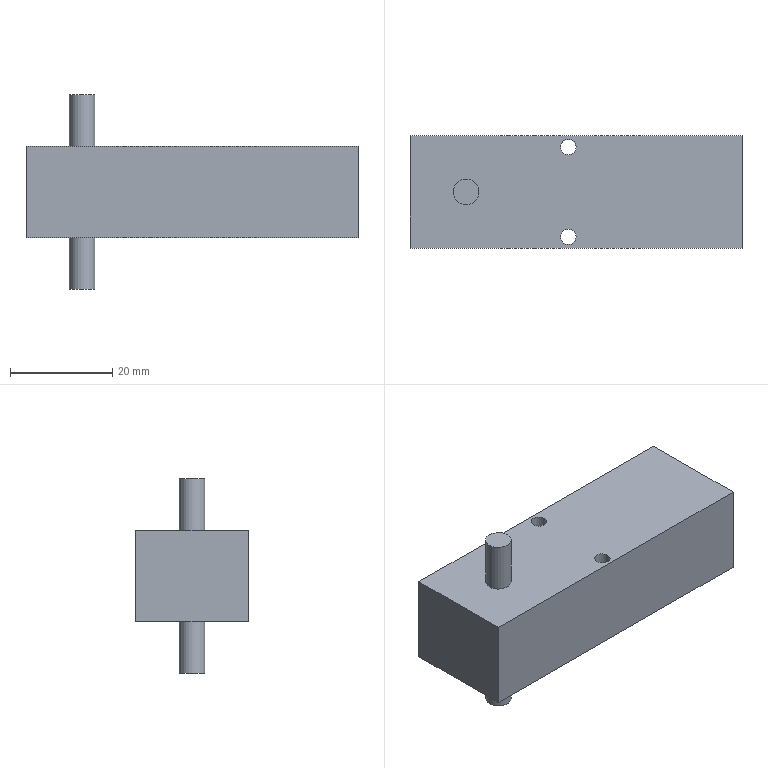Part | NX | features BREP 1 | 1 solid | 12 faces | box 65 x 22 x 38 mm | volume 25878 mm3 | plane 8 | cylinder 4 | commonest cylinder face diameters 3 x2 5 x2
STEP:
#1=CARTESIAN_POINT('',(-3.,-8.8,9.));
#2=VERTEX_POINT('',#1);
#3=CARTESIAN_POINT('',(-1.5,-8.8,9.));
#4=DIRECTION('',(0.,0.,1.));
#5=DIRECTION('',(-1.,0.,0.));
#6=AXIS2_PLACEMENT_3D('',#3,#4,#5);
#7=CIRCLE('',#6,1.5);
#8=EDGE_CURVE('',#2,#2,#7,.T.);
#9=ORIENTED_EDGE('',*,*,#8,.T.);
#10=EDGE_LOOP('',(#9));
#11=FACE_BOUND('',#10,.T.);
#12=CARTESIAN_POINT('',(0.,-8.8,-9.));
#13=VERTEX_POINT('',#12);
#14=CARTESIAN_POINT('',(-1.5,-8.8,-9.));
#15=DIRECTION('',(0.,0.,-1.));
#16=DIRECTION('',(1.,0.,0.));
#17=AXIS2_PLACEMENT_3D('',#14,#15,#16);
#18=CIRCLE('',#17,1.5);
#19=EDGE_CURVE('',#13,#13,#18,.T.);
#20=ORIENTED_EDGE('',*,*,#19,.T.);
#21=EDGE_LOOP('',(#20));
#22=FACE_BOUND('',#21,.T.);
#23=CARTESIAN_POINT('',(-1.5,-8.8,-13.243));
#24=DIRECTION('',(0.,0.,1.));
#25=DIRECTION('',(-1.,0.,0.));
#26=AXIS2_PLACEMENT_3D('',#23,#24,#25);
#27=CYLINDRICAL_SURFACE('',#26,1.5);
#28=ADVANCED_FACE('',(#11,#22),#27,.F.);
#29=CARTESIAN_POINT('',(0.,8.8,9.));
#30=VERTEX_POINT('',#29);
#31=CARTESIAN_POINT('',(-1.5,8.8,9.));
#32=DIRECTION('',(0.,0.,1.));
#33=DIRECTION('',(1.,0.,0.));
#34=AXIS2_PLACEMENT_3D('',#31,#32,#33);
#35=CIRCLE('',#34,1.5);
#36=EDGE_CURVE('',#30,#30,#35,.T.);
#37=ORIENTED_EDGE('',*,*,#36,.T.);
#38=EDGE_LOOP('',(#37));
#39=FACE_BOUND('',#38,.T.);
#40=CARTESIAN_POINT('',(0.,8.8,-9.));
#41=VERTEX_POINT('',#40);
#42=CARTESIAN_POINT('',(-1.5,8.8,-9.));
#43=DIRECTION('',(0.,0.,-1.));
#44=DIRECTION('',(1.,0.,0.));
#45=AXIS2_PLACEMENT_3D('',#42,#43,#44);
#46=CIRCLE('',#45,1.5);
#47=EDGE_CURVE('',#41,#41,#46,.T.);
#48=ORIENTED_EDGE('',*,*,#47,.T.);
#49=EDGE_LOOP('',(#48));
#50=FACE_BOUND('',#49,.T.);
#51=CARTESIAN_POINT('',(-1.5,8.8,-13.243));
#52=DIRECTION('',(0.,0.,1.));
#53=DIRECTION('',(-1.,0.,0.));
#54=AXIS2_PLACEMENT_3D('',#51,#52,#53);
#55=CYLINDRICAL_SURFACE('',#54,1.5);
#56=ADVANCED_FACE('',(#39,#50),#55,.F.);
#57=CARTESIAN_POINT('',(-19.,0.,-9.));
#58=VERTEX_POINT('',#57);
#59=CARTESIAN_POINT('',(-21.5,0.,-9.));
#60=DIRECTION('',(0.,0.,1.));
#61=DIRECTION('',(1.,0.,0.));
#62=AXIS2_PLACEMENT_3D('',#59,#60,#61);
#63=CIRCLE('',#62,2.5);
#64=EDGE_CURVE('',#58,#58,#63,.T.);
#65=ORIENTED_EDGE('',*,*,#64,.F.);
#66=EDGE_LOOP('',(#65));
#67=FACE_BOUND('',#66,.T.);
#68=CARTESIAN_POINT('',(-19.,0.,-19.));
#69=VERTEX_POINT('',#68);
#70=CARTESIAN_POINT('',(-21.5,0.,-19.));
#71=DIRECTION('',(0.,0.,1.));
#72=DIRECTION('',(1.,0.,0.));
#73=AXIS2_PLACEMENT_3D('',#70,#71,#72);
#74=CIRCLE('',#73,2.5);
#75=EDGE_CURVE('',#69,#69,#74,.T.);
#76=ORIENTED_EDGE('',*,*,#75,.T.);
#77=EDGE_LOOP('',(#76));
#78=FACE_BOUND('',#77,.T.);
#79=CARTESIAN_POINT('',(-21.5,0.,-19.));
#80=DIRECTION('',(0.,0.,1.));
#81=DIRECTION('',(-1.,0.,0.));
#82=AXIS2_PLACEMENT_3D('',#79,#80,#81);
#83=CYLINDRICAL_SURFACE('',#82,2.5);
#84=ADVANCED_FACE('',(#67,#78),#83,.T.);
#85=CARTESIAN_POINT('',(-19.,0.,9.));
#86=VERTEX_POINT('',#85);
#87=CARTESIAN_POINT('',(-21.5,0.,9.));
#88=DIRECTION('',(0.,0.,1.));
#89=DIRECTION('',(1.,0.,0.));
#90=AXIS2_PLACEMENT_3D('',#87,#88,#89);
#91=CIRCLE('',#90,2.5);
#92=EDGE_CURVE('',#86,#86,#91,.T.);
#93=ORIENTED_EDGE('',*,*,#92,.T.);
#94=EDGE_LOOP('',(#93));
#95=FACE_BOUND('',#94,.T.);
#96=CARTESIAN_POINT('',(-19.,0.,19.));
#97=VERTEX_POINT('',#96);
#98=CARTESIAN_POINT('',(-21.5,0.,19.));
#99=DIRECTION('',(0.,0.,1.));
#100=DIRECTION('',(1.,0.,0.));
#101=AXIS2_PLACEMENT_3D('',#98,#99,#100);
#102=CIRCLE('',#101,2.5);
#103=EDGE_CURVE('',#97,#97,#102,.T.);
#104=ORIENTED_EDGE('',*,*,#103,.F.);
#105=EDGE_LOOP('',(#104));
#106=FACE_BOUND('',#105,.T.);
#107=CARTESIAN_POINT('',(-21.5,0.,19.));
#108=DIRECTION('',(0.,0.,-1.));
#109=DIRECTION('',(1.,0.,0.));
#110=AXIS2_PLACEMENT_3D('',#107,#108,#109);
#111=CYLINDRICAL_SURFACE('',#110,2.5);
#112=ADVANCED_FACE('',(#95,#106),#111,.T.);
#113=ORIENTED_EDGE('',*,*,#8,.F.);
#114=EDGE_LOOP('',(#113));
#115=FACE_BOUND('',#114,.T.);
#116=ORIENTED_EDGE('',*,*,#36,.F.);
#117=EDGE_LOOP('',(#116));
#118=FACE_BOUND('',#117,.T.);
#119=CARTESIAN_POINT('',(32.5,-11.,9.));
#120=VERTEX_POINT('',#119);
#121=CARTESIAN_POINT('',(32.5,11.,9.));
#122=VERTEX_POINT('',#121);
#123=CARTESIAN_POINT('',(32.5,11.,9.));
#124=DIRECTION('',(0.,1.,0.));
#125=VECTOR('',#124,1000.);
#126=LINE('',#123,#125);
#127=EDGE_CURVE('',#120,#122,#126,.T.);
#128=ORIENTED_EDGE('',*,*,#127,.T.);
#129=CARTESIAN_POINT('',(-32.5,11.,9.));
#130=VERTEX_POINT('',#129);
#131=CARTESIAN_POINT('',(-32.5,11.,9.));
#132=DIRECTION('',(-1.,0.,0.));
#133=VECTOR('',#132,1000.);
#134=LINE('',#131,#133);
#135=EDGE_CURVE('',#122,#130,#134,.T.);
#136=ORIENTED_EDGE('',*,*,#135,.T.);
#137=CARTESIAN_POINT('',(-32.5,-11.,9.));
#138=VERTEX_POINT('',#137);
#139=CARTESIAN_POINT('',(-32.5,11.,9.));
#140=DIRECTION('',(0.,-1.,0.));
#141=VECTOR('',#140,1000.);
#142=LINE('',#139,#141);
#143=EDGE_CURVE('',#130,#138,#142,.T.);
#144=ORIENTED_EDGE('',*,*,#143,.T.);
#145=CARTESIAN_POINT('',(-32.5,-11.,9.));
#146=DIRECTION('',(1.,0.,0.));
#147=VECTOR('',#146,1000.);
#148=LINE('',#145,#147);
#149=EDGE_CURVE('',#138,#120,#148,.T.);
#150=ORIENTED_EDGE('',*,*,#149,.T.);
#151=EDGE_LOOP('',(#128,#136,#144,#150));
#152=FACE_BOUND('',#151,.T.);
#153=ORIENTED_EDGE('',*,*,#92,.F.);
#154=EDGE_LOOP('',(#153));
#155=FACE_BOUND('',#154,.T.);
#156=CARTESIAN_POINT('',(0.,0.,9.));
#157=DIRECTION('',(0.,0.,1.));
#158=DIRECTION('',(-1.,0.,0.));
#159=AXIS2_PLACEMENT_3D('',#156,#157,#158);
#160=PLANE('',#159);
#161=ADVANCED_FACE('',(#115,#118,#152,#155),#160,.T.);
#162=CARTESIAN_POINT('',(32.5,-11.,-9.));
#163=VERTEX_POINT('',#162);
#164=CARTESIAN_POINT('',(32.5,11.,-9.));
#165=VERTEX_POINT('',#164);
#166=CARTESIAN_POINT('',(32.5,11.,-9.));
#167=DIRECTION('',(0.,1.,0.));
#168=VECTOR('',#167,1000.);
#169=LINE('',#166,#168);
#170=EDGE_CURVE('',#163,#165,#169,.T.);
#171=ORIENTED_EDGE('',*,*,#170,.T.);
#172=CARTESIAN_POINT('',(32.5,11.,9.));
#173=DIRECTION('',(0.,0.,-1.));
#174=VECTOR('',#173,1000.);
#175=LINE('',#172,#174);
#176=EDGE_CURVE('',#122,#165,#175,.T.);
#177=ORIENTED_EDGE('',*,*,#176,.F.);
#178=ORIENTED_EDGE('',*,*,#127,.F.);
#179=CARTESIAN_POINT('',(32.5,-11.,9.));
#180=DIRECTION('',(0.,0.,-1.));
#181=VECTOR('',#180,1000.);
#182=LINE('',#179,#181);
#183=EDGE_CURVE('',#120,#163,#182,.T.);
#184=ORIENTED_EDGE('',*,*,#183,.T.);
#185=EDGE_LOOP('',(#171,#177,#178,#184));
#186=FACE_BOUND('',#185,.T.);
#187=CARTESIAN_POINT('',(32.5,11.,9.));
#188=DIRECTION('',(-1.,0.,0.));
#189=DIRECTION('',(0.,1.,0.));
#190=AXIS2_PLACEMENT_3D('',#187,#188,#189);
#191=PLANE('',#190);
#192=ADVANCED_FACE('',(#186),#191,.F.);
#193=CARTESIAN_POINT('',(-32.5,11.,-9.));
#194=VERTEX_POINT('',#193);
#195=CARTESIAN_POINT('',(-32.5,11.,-9.));
#196=DIRECTION('',(-1.,0.,0.));
#197=VECTOR('',#196,1000.);
#198=LINE('',#195,#197);
#199=EDGE_CURVE('',#165,#194,#198,.T.);
#200=ORIENTED_EDGE('',*,*,#199,.T.);
#201=CARTESIAN_POINT('',(-32.5,11.,9.));
#202=DIRECTION('',(0.,0.,-1.));
#203=VECTOR('',#202,1000.);
#204=LINE('',#201,#203);
#205=EDGE_CURVE('',#130,#194,#204,.T.);
#206=ORIENTED_EDGE('',*,*,#205,.F.);
#207=ORIENTED_EDGE('',*,*,#135,.F.);
#208=ORIENTED_EDGE('',*,*,#176,.T.);
#209=EDGE_LOOP('',(#200,#206,#207,#208));
#210=FACE_BOUND('',#209,.T.);
#211=CARTESIAN_POINT('',(-32.5,11.,9.));
#212=DIRECTION('',(0.,-1.,0.));
#213=DIRECTION('',(0.,0.,1.));
#214=AXIS2_PLACEMENT_3D('',#211,#212,#213);
#215=PLANE('',#214);
#216=ADVANCED_FACE('',(#210),#215,.F.);
#217=CARTESIAN_POINT('',(-32.5,-11.,-9.));
#218=VERTEX_POINT('',#217);
#219=CARTESIAN_POINT('',(-32.5,11.,-9.));
#220=DIRECTION('',(0.,-1.,0.));
#221=VECTOR('',#220,1000.);
#222=LINE('',#219,#221);
#223=EDGE_CURVE('',#194,#218,#222,.T.);
#224=ORIENTED_EDGE('',*,*,#223,.T.);
#225=CARTESIAN_POINT('',(-32.5,-11.,9.));
#226=DIRECTION('',(0.,0.,-1.));
#227=VECTOR('',#226,1000.);
#228=LINE('',#225,#227);
#229=EDGE_CURVE('',#138,#218,#228,.T.);
#230=ORIENTED_EDGE('',*,*,#229,.F.);
#231=ORIENTED_EDGE('',*,*,#143,.F.);
#232=ORIENTED_EDGE('',*,*,#205,.T.);
#233=EDGE_LOOP('',(#224,#230,#231,#232));
#234=FACE_BOUND('',#233,.T.);
#235=CARTESIAN_POINT('',(-32.5,11.,9.));
#236=DIRECTION('',(1.,0.,0.));
#237=DIRECTION('',(0.,0.,1.));
#238=AXIS2_PLACEMENT_3D('',#235,#236,#237);
#239=PLANE('',#238);
#240=ADVANCED_FACE('',(#234),#239,.F.);
#241=CARTESIAN_POINT('',(-32.5,-11.,-9.));
#242=DIRECTION('',(1.,0.,0.));
#243=VECTOR('',#242,1000.);
#244=LINE('',#241,#243);
#245=EDGE_CURVE('',#218,#163,#244,.T.);
#246=ORIENTED_EDGE('',*,*,#245,.T.);
#247=ORIENTED_EDGE('',*,*,#183,.F.);
#248=ORIENTED_EDGE('',*,*,#149,.F.);
#249=ORIENTED_EDGE('',*,*,#229,.T.);
#250=EDGE_LOOP('',(#246,#247,#248,#249));
#251=FACE_BOUND('',#250,.T.);
#252=CARTESIAN_POINT('',(-32.5,-11.,9.));
#253=DIRECTION('',(0.,1.,0.));
#254=DIRECTION('',(0.,0.,-1.));
#255=AXIS2_PLACEMENT_3D('',#252,#253,#254);
#256=PLANE('',#255);
#257=ADVANCED_FACE('',(#251),#256,.F.);
#258=ORIENTED_EDGE('',*,*,#19,.F.);
#259=EDGE_LOOP('',(#258));
#260=FACE_BOUND('',#259,.T.);
#261=ORIENTED_EDGE('',*,*,#47,.F.);
#262=EDGE_LOOP('',(#261));
#263=FACE_BOUND('',#262,.T.);
#264=ORIENTED_EDGE('',*,*,#64,.T.);
#265=EDGE_LOOP('',(#264));
#266=FACE_BOUND('',#265,.T.);
#267=ORIENTED_EDGE('',*,*,#170,.F.);
#268=ORIENTED_EDGE('',*,*,#245,.F.);
#269=ORIENTED_EDGE('',*,*,#223,.F.);
#270=ORIENTED_EDGE('',*,*,#199,.F.);
#271=EDGE_LOOP('',(#267,#268,#269,#270));
#272=FACE_BOUND('',#271,.T.);
#273=CARTESIAN_POINT('',(0.,0.,-9.));
#274=DIRECTION('',(0.,0.,1.));
#275=DIRECTION('',(-1.,0.,0.));
#276=AXIS2_PLACEMENT_3D('',#273,#274,#275);
#277=PLANE('',#276);
#278=ADVANCED_FACE('',(#260,#263,#266,#272),#277,.F.);
#279=ORIENTED_EDGE('',*,*,#103,.T.);
#280=EDGE_LOOP('',(#279));
#281=FACE_BOUND('',#280,.T.);
#282=CARTESIAN_POINT('',(-21.5,0.,19.));
#283=DIRECTION('',(0.,0.,1.));
#284=DIRECTION('',(-1.,0.,0.));
#285=AXIS2_PLACEMENT_3D('',#282,#283,#284);
#286=PLANE('',#285);
#287=ADVANCED_FACE('',(#281),#286,.T.);
#288=ORIENTED_EDGE('',*,*,#75,.F.);
#289=EDGE_LOOP('',(#288));
#290=FACE_BOUND('',#289,.T.);
#291=CARTESIAN_POINT('',(-21.5,0.,-19.));
#292=DIRECTION('',(0.,0.,-1.));
#293=DIRECTION('',(-1.,0.,0.));
#294=AXIS2_PLACEMENT_3D('',#291,#292,#293);
#295=PLANE('',#294);
#296=ADVANCED_FACE('',(#290),#295,.T.);
#297=CLOSED_SHELL('',(#28,#56,#84,#112,#161,#192,#216,#240,#257,#278,#287,#296));
#298=MANIFOLD_SOLID_BREP('',#297);
#299=(LENGTH_UNIT()NAMED_UNIT(*)SI_UNIT(.MILLI.,.METRE.));
#300=UNCERTAINTY_MEASURE_WITH_UNIT(LENGTH_MEASURE(0.00001),#299,'','');
#301=(NAMED_UNIT(*)PLANE_ANGLE_UNIT()SI_UNIT($,.RADIAN.));
#302=(NAMED_UNIT(*)SI_UNIT($,.STERADIAN.)SOLID_ANGLE_UNIT());
#303=(GEOMETRIC_REPRESENTATION_CONTEXT(3)GLOBAL_UNCERTAINTY_ASSIGNED_CONTEXT((#300))GLOBAL_UNIT_ASSIGNED_CONTEXT((#299,#301,#302))REPRESENTATION_CONTEXT('',''));
#304=ADVANCED_BREP_SHAPE_REPRESENTATION('',(#298),#303);